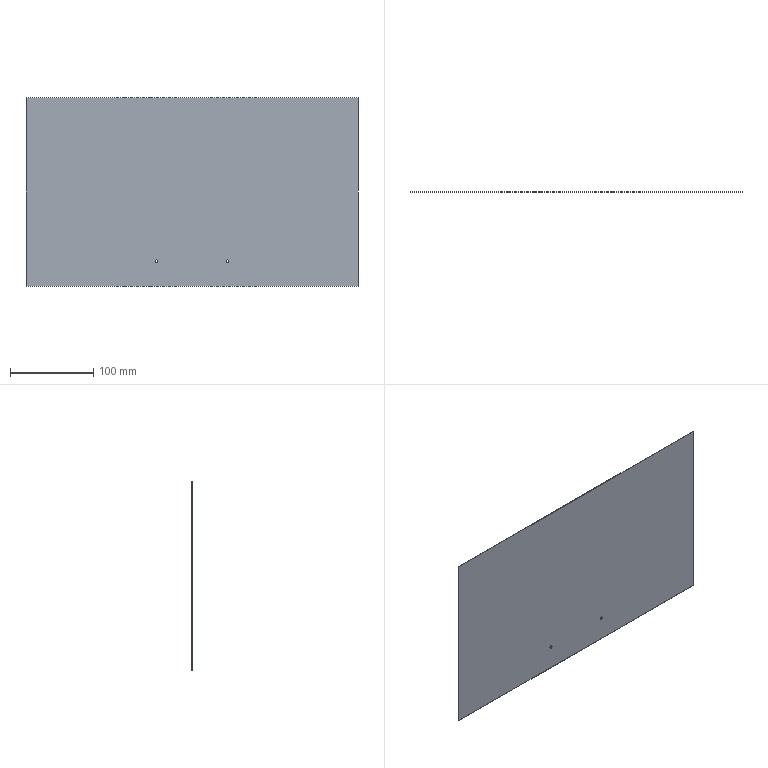Part | SolidWorks | features 3DProfileFeature 1, FlatPattern 1, HoleWzd 1, SMBaseFlange 1, SheetMetal 1 | 1 solid | 10 faces | box 398 x 0.5 x 226 mm | volume 44966 mm3 | plane 6 | cylinder 4 | commonest cylinder face diameters 3.2 x4
STEP:
#1=CARTESIAN_POINT('',(156.5,0.,-194.4));
#2=VERTEX_POINT('',#1);
#3=CARTESIAN_POINT('',(156.5,0.,-197.6));
#4=VERTEX_POINT('',#3);
#5=CARTESIAN_POINT('',(156.5,0.,-196.));
#6=DIRECTION('',(0.,-1.,0.));
#7=DIRECTION('',(0.,0.,-1.));
#8=AXIS2_PLACEMENT_3D('',#5,#6,#7);
#9=CIRCLE('',#8,1.6);
#10=EDGE_CURVE('',#2,#4,#9,.T.);
#11=ORIENTED_EDGE('',*,*,#10,.T.);
#12=CARTESIAN_POINT('',(156.5,0.5,-197.6));
#13=VERTEX_POINT('',#12);
#14=CARTESIAN_POINT('',(156.5,0.5,-197.6));
#15=DIRECTION('',(0.,1.,0.));
#16=VECTOR('',#15,1000.);
#17=LINE('',#14,#16);
#18=EDGE_CURVE('',#4,#13,#17,.T.);
#19=ORIENTED_EDGE('',*,*,#18,.T.);
#20=CARTESIAN_POINT('',(156.5,0.5,-194.4));
#21=VERTEX_POINT('',#20);
#22=CARTESIAN_POINT('',(156.5,0.5,-196.));
#23=DIRECTION('',(0.,1.,0.));
#24=DIRECTION('',(0.,0.,1.));
#25=AXIS2_PLACEMENT_3D('',#22,#23,#24);
#26=CIRCLE('',#25,1.6);
#27=EDGE_CURVE('',#13,#21,#26,.T.);
#28=ORIENTED_EDGE('',*,*,#27,.T.);
#29=CARTESIAN_POINT('',(156.5,0.5,-194.4));
#30=DIRECTION('',(0.,1.,0.));
#31=VECTOR('',#30,1000.);
#32=LINE('',#29,#31);
#33=EDGE_CURVE('',#2,#21,#32,.T.);
#34=ORIENTED_EDGE('',*,*,#33,.F.);
#35=EDGE_LOOP('',(#11,#19,#28,#34));
#36=FACE_OUTER_BOUND('',#35,.T.);
#37=CARTESIAN_POINT('',(156.5,0.5,-196.));
#38=DIRECTION('',(0.,1.,0.));
#39=DIRECTION('',(0.,0.,1.));
#40=AXIS2_PLACEMENT_3D('',#37,#38,#39);
#41=CYLINDRICAL_SURFACE('',#40,1.6);
#42=ADVANCED_FACE('',(#36),#41,.F.);
#43=CARTESIAN_POINT('',(241.5,0.,-194.4));
#44=VERTEX_POINT('',#43);
#45=CARTESIAN_POINT('',(241.5,0.,-197.6));
#46=VERTEX_POINT('',#45);
#47=CARTESIAN_POINT('',(241.5,0.,-196.));
#48=DIRECTION('',(0.,-1.,0.));
#49=DIRECTION('',(0.,0.,-1.));
#50=AXIS2_PLACEMENT_3D('',#47,#48,#49);
#51=CIRCLE('',#50,1.6);
#52=EDGE_CURVE('',#44,#46,#51,.T.);
#53=ORIENTED_EDGE('',*,*,#52,.T.);
#54=CARTESIAN_POINT('',(241.5,0.5,-197.6));
#55=VERTEX_POINT('',#54);
#56=CARTESIAN_POINT('',(241.5,0.5,-197.6));
#57=DIRECTION('',(0.,1.,0.));
#58=VECTOR('',#57,1000.);
#59=LINE('',#56,#58);
#60=EDGE_CURVE('',#46,#55,#59,.T.);
#61=ORIENTED_EDGE('',*,*,#60,.T.);
#62=CARTESIAN_POINT('',(241.5,0.5,-194.4));
#63=VERTEX_POINT('',#62);
#64=CARTESIAN_POINT('',(241.5,0.5,-196.));
#65=DIRECTION('',(0.,1.,0.));
#66=DIRECTION('',(0.,0.,1.));
#67=AXIS2_PLACEMENT_3D('',#64,#65,#66);
#68=CIRCLE('',#67,1.6);
#69=EDGE_CURVE('',#55,#63,#68,.T.);
#70=ORIENTED_EDGE('',*,*,#69,.T.);
#71=CARTESIAN_POINT('',(241.5,0.5,-194.4));
#72=DIRECTION('',(0.,1.,0.));
#73=VECTOR('',#72,1000.);
#74=LINE('',#71,#73);
#75=EDGE_CURVE('',#44,#63,#74,.T.);
#76=ORIENTED_EDGE('',*,*,#75,.F.);
#77=EDGE_LOOP('',(#53,#61,#70,#76));
#78=FACE_OUTER_BOUND('',#77,.T.);
#79=CARTESIAN_POINT('',(241.5,0.5,-196.));
#80=DIRECTION('',(0.,1.,0.));
#81=DIRECTION('',(0.,0.,1.));
#82=AXIS2_PLACEMENT_3D('',#79,#80,#81);
#83=CYLINDRICAL_SURFACE('',#82,1.6);
#84=ADVANCED_FACE('',(#78),#83,.F.);
#85=CARTESIAN_POINT('',(0.,0.,-226.));
#86=VERTEX_POINT('',#85);
#87=CARTESIAN_POINT('',(0.,0.,0.));
#88=VERTEX_POINT('',#87);
#89=CARTESIAN_POINT('',(0.,0.,0.));
#90=DIRECTION('',(0.,0.,1.));
#91=VECTOR('',#90,1000.);
#92=LINE('',#89,#91);
#93=EDGE_CURVE('',#86,#88,#92,.T.);
#94=ORIENTED_EDGE('',*,*,#93,.T.);
#95=CARTESIAN_POINT('',(0.,0.5,0.));
#96=VERTEX_POINT('',#95);
#97=CARTESIAN_POINT('',(0.,0.5,0.));
#98=DIRECTION('',(0.,-1.,0.));
#99=VECTOR('',#98,1000.);
#100=LINE('',#97,#99);
#101=EDGE_CURVE('',#96,#88,#100,.T.);
#102=ORIENTED_EDGE('',*,*,#101,.F.);
#103=CARTESIAN_POINT('',(0.,0.5,-226.));
#104=VERTEX_POINT('',#103);
#105=CARTESIAN_POINT('',(0.,0.5,0.));
#106=DIRECTION('',(0.,0.,1.));
#107=VECTOR('',#106,1000.);
#108=LINE('',#105,#107);
#109=EDGE_CURVE('',#104,#96,#108,.T.);
#110=ORIENTED_EDGE('',*,*,#109,.F.);
#111=CARTESIAN_POINT('',(0.,0.5,-226.));
#112=DIRECTION('',(0.,-1.,0.));
#113=VECTOR('',#112,1000.);
#114=LINE('',#111,#113);
#115=EDGE_CURVE('',#104,#86,#114,.T.);
#116=ORIENTED_EDGE('',*,*,#115,.T.);
#117=EDGE_LOOP('',(#94,#102,#110,#116));
#118=FACE_OUTER_BOUND('',#117,.T.);
#119=CARTESIAN_POINT('',(0.,0.5,0.));
#120=DIRECTION('',(1.,0.,0.));
#121=DIRECTION('',(0.,0.,-1.));
#122=AXIS2_PLACEMENT_3D('',#119,#120,#121);
#123=PLANE('',#122);
#124=ADVANCED_FACE('',(#118),#123,.F.);
#125=CARTESIAN_POINT('',(398.,0.,0.));
#126=VERTEX_POINT('',#125);
#127=CARTESIAN_POINT('',(0.,0.,0.));
#128=DIRECTION('',(1.,0.,0.));
#129=VECTOR('',#128,1000.);
#130=LINE('',#127,#129);
#131=EDGE_CURVE('',#88,#126,#130,.T.);
#132=ORIENTED_EDGE('',*,*,#131,.T.);
#133=CARTESIAN_POINT('',(398.,0.5,0.));
#134=VERTEX_POINT('',#133);
#135=CARTESIAN_POINT('',(398.,0.5,0.));
#136=DIRECTION('',(0.,-1.,0.));
#137=VECTOR('',#136,1000.);
#138=LINE('',#135,#137);
#139=EDGE_CURVE('',#134,#126,#138,.T.);
#140=ORIENTED_EDGE('',*,*,#139,.F.);
#141=CARTESIAN_POINT('',(0.,0.5,0.));
#142=DIRECTION('',(1.,0.,0.));
#143=VECTOR('',#142,1000.);
#144=LINE('',#141,#143);
#145=EDGE_CURVE('',#96,#134,#144,.T.);
#146=ORIENTED_EDGE('',*,*,#145,.F.);
#147=ORIENTED_EDGE('',*,*,#101,.T.);
#148=EDGE_LOOP('',(#132,#140,#146,#147));
#149=FACE_OUTER_BOUND('',#148,.T.);
#150=CARTESIAN_POINT('',(0.,0.5,0.));
#151=DIRECTION('',(0.,0.,-1.));
#152=DIRECTION('',(-1.,0.,0.));
#153=AXIS2_PLACEMENT_3D('',#150,#151,#152);
#154=PLANE('',#153);
#155=ADVANCED_FACE('',(#149),#154,.F.);
#156=CARTESIAN_POINT('',(398.,0.,-226.));
#157=VERTEX_POINT('',#156);
#158=CARTESIAN_POINT('',(398.,0.,0.));
#159=DIRECTION('',(0.,0.,-1.));
#160=VECTOR('',#159,1000.);
#161=LINE('',#158,#160);
#162=EDGE_CURVE('',#126,#157,#161,.T.);
#163=ORIENTED_EDGE('',*,*,#162,.T.);
#164=CARTESIAN_POINT('',(398.,0.5,-226.));
#165=VERTEX_POINT('',#164);
#166=CARTESIAN_POINT('',(398.,0.5,-226.));
#167=DIRECTION('',(0.,-1.,0.));
#168=VECTOR('',#167,1000.);
#169=LINE('',#166,#168);
#170=EDGE_CURVE('',#165,#157,#169,.T.);
#171=ORIENTED_EDGE('',*,*,#170,.F.);
#172=CARTESIAN_POINT('',(398.,0.5,0.));
#173=DIRECTION('',(0.,0.,-1.));
#174=VECTOR('',#173,1000.);
#175=LINE('',#172,#174);
#176=EDGE_CURVE('',#134,#165,#175,.T.);
#177=ORIENTED_EDGE('',*,*,#176,.F.);
#178=ORIENTED_EDGE('',*,*,#139,.T.);
#179=EDGE_LOOP('',(#163,#171,#177,#178));
#180=FACE_OUTER_BOUND('',#179,.T.);
#181=CARTESIAN_POINT('',(398.,0.5,0.));
#182=DIRECTION('',(-1.,0.,0.));
#183=DIRECTION('',(0.,0.,1.));
#184=AXIS2_PLACEMENT_3D('',#181,#182,#183);
#185=PLANE('',#184);
#186=ADVANCED_FACE('',(#180),#185,.F.);
#187=CARTESIAN_POINT('',(0.,0.,-226.));
#188=DIRECTION('',(-1.,0.,0.));
#189=VECTOR('',#188,1000.);
#190=LINE('',#187,#189);
#191=EDGE_CURVE('',#157,#86,#190,.T.);
#192=ORIENTED_EDGE('',*,*,#191,.T.);
#193=ORIENTED_EDGE('',*,*,#115,.F.);
#194=CARTESIAN_POINT('',(0.,0.5,-226.));
#195=DIRECTION('',(-1.,0.,0.));
#196=VECTOR('',#195,1000.);
#197=LINE('',#194,#196);
#198=EDGE_CURVE('',#165,#104,#197,.T.);
#199=ORIENTED_EDGE('',*,*,#198,.F.);
#200=ORIENTED_EDGE('',*,*,#170,.T.);
#201=EDGE_LOOP('',(#192,#193,#199,#200));
#202=FACE_OUTER_BOUND('',#201,.T.);
#203=CARTESIAN_POINT('',(0.,0.5,-226.));
#204=DIRECTION('',(0.,0.,1.));
#205=DIRECTION('',(1.,0.,0.));
#206=AXIS2_PLACEMENT_3D('',#203,#204,#205);
#207=PLANE('',#206);
#208=ADVANCED_FACE('',(#202),#207,.F.);
#209=CARTESIAN_POINT('',(156.5,0.5,-196.));
#210=DIRECTION('',(0.,1.,0.));
#211=DIRECTION('',(0.,0.,1.));
#212=AXIS2_PLACEMENT_3D('',#209,#210,#211);
#213=CIRCLE('',#212,1.6);
#214=EDGE_CURVE('',#21,#13,#213,.T.);
#215=ORIENTED_EDGE('',*,*,#214,.F.);
#216=ORIENTED_EDGE('',*,*,#27,.F.);
#217=EDGE_LOOP('',(#215,#216));
#218=FACE_BOUND('',#217,.T.);
#219=CARTESIAN_POINT('',(241.5,0.5,-196.));
#220=DIRECTION('',(0.,1.,0.));
#221=DIRECTION('',(0.,0.,1.));
#222=AXIS2_PLACEMENT_3D('',#219,#220,#221);
#223=CIRCLE('',#222,1.6);
#224=EDGE_CURVE('',#63,#55,#223,.T.);
#225=ORIENTED_EDGE('',*,*,#224,.F.);
#226=ORIENTED_EDGE('',*,*,#69,.F.);
#227=EDGE_LOOP('',(#225,#226));
#228=FACE_BOUND('',#227,.T.);
#229=ORIENTED_EDGE('',*,*,#109,.T.);
#230=ORIENTED_EDGE('',*,*,#145,.T.);
#231=ORIENTED_EDGE('',*,*,#176,.T.);
#232=ORIENTED_EDGE('',*,*,#198,.T.);
#233=EDGE_LOOP('',(#229,#230,#231,#232));
#234=FACE_OUTER_BOUND('',#233,.T.);
#235=CARTESIAN_POINT('',(0.,0.5,-226.));
#236=DIRECTION('',(0.,-1.,0.));
#237=DIRECTION('',(0.,0.,-1.));
#238=AXIS2_PLACEMENT_3D('',#235,#236,#237);
#239=PLANE('',#238);
#240=ADVANCED_FACE('',(#218,#228,#234),#239,.F.);
#241=ORIENTED_EDGE('',*,*,#10,.F.);
#242=CARTESIAN_POINT('',(156.5,0.,-196.));
#243=DIRECTION('',(0.,-1.,0.));
#244=DIRECTION('',(0.,0.,-1.));
#245=AXIS2_PLACEMENT_3D('',#242,#243,#244);
#246=CIRCLE('',#245,1.6);
#247=EDGE_CURVE('',#4,#2,#246,.T.);
#248=ORIENTED_EDGE('',*,*,#247,.F.);
#249=EDGE_LOOP('',(#241,#248));
#250=FACE_BOUND('',#249,.T.);
#251=ORIENTED_EDGE('',*,*,#52,.F.);
#252=CARTESIAN_POINT('',(241.5,0.,-196.));
#253=DIRECTION('',(0.,-1.,0.));
#254=DIRECTION('',(0.,0.,-1.));
#255=AXIS2_PLACEMENT_3D('',#252,#253,#254);
#256=CIRCLE('',#255,1.6);
#257=EDGE_CURVE('',#46,#44,#256,.T.);
#258=ORIENTED_EDGE('',*,*,#257,.F.);
#259=EDGE_LOOP('',(#251,#258));
#260=FACE_BOUND('',#259,.T.);
#261=ORIENTED_EDGE('',*,*,#93,.F.);
#262=ORIENTED_EDGE('',*,*,#191,.F.);
#263=ORIENTED_EDGE('',*,*,#162,.F.);
#264=ORIENTED_EDGE('',*,*,#131,.F.);
#265=EDGE_LOOP('',(#261,#262,#263,#264));
#266=FACE_OUTER_BOUND('',#265,.T.);
#267=CARTESIAN_POINT('',(0.,0.,-226.));
#268=DIRECTION('',(0.,-1.,0.));
#269=DIRECTION('',(0.,0.,-1.));
#270=AXIS2_PLACEMENT_3D('',#267,#268,#269);
#271=PLANE('',#270);
#272=ADVANCED_FACE('',(#250,#260,#266),#271,.T.);
#273=ORIENTED_EDGE('',*,*,#60,.F.);
#274=ORIENTED_EDGE('',*,*,#257,.T.);
#275=ORIENTED_EDGE('',*,*,#75,.T.);
#276=ORIENTED_EDGE('',*,*,#224,.T.);
#277=EDGE_LOOP('',(#273,#274,#275,#276));
#278=FACE_OUTER_BOUND('',#277,.T.);
#279=CARTESIAN_POINT('',(241.5,0.5,-196.));
#280=DIRECTION('',(0.,1.,0.));
#281=DIRECTION('',(0.,0.,1.));
#282=AXIS2_PLACEMENT_3D('',#279,#280,#281);
#283=CYLINDRICAL_SURFACE('',#282,1.6);
#284=ADVANCED_FACE('',(#278),#283,.F.);
#285=ORIENTED_EDGE('',*,*,#18,.F.);
#286=ORIENTED_EDGE('',*,*,#247,.T.);
#287=ORIENTED_EDGE('',*,*,#33,.T.);
#288=ORIENTED_EDGE('',*,*,#214,.T.);
#289=EDGE_LOOP('',(#285,#286,#287,#288));
#290=FACE_OUTER_BOUND('',#289,.T.);
#291=CARTESIAN_POINT('',(156.5,0.5,-196.));
#292=DIRECTION('',(0.,1.,0.));
#293=DIRECTION('',(0.,0.,1.));
#294=AXIS2_PLACEMENT_3D('',#291,#292,#293);
#295=CYLINDRICAL_SURFACE('',#294,1.6);
#296=ADVANCED_FACE('',(#290),#295,.F.);
#297=CLOSED_SHELL('',(#42,#84,#124,#155,#186,#208,#240,#272,#284,#296));
#298=MANIFOLD_SOLID_BREP('',#297);
#299=CARTESIAN_POINT('',(0.,0.,0.));
#300=DIRECTION('',(0.,0.,1.));
#301=DIRECTION('',(1.,0.,0.));
#302=AXIS2_PLACEMENT_3D('',#299,#300,#301);
#303=(LENGTH_UNIT()NAMED_UNIT(*)SI_UNIT(.MILLI.,.METRE.));
#304=UNCERTAINTY_MEASURE_WITH_UNIT(LENGTH_MEASURE(0.00001),#303,'','');
#305=(NAMED_UNIT(*)PLANE_ANGLE_UNIT()SI_UNIT($,.RADIAN.));
#306=(NAMED_UNIT(*)SI_UNIT($,.STERADIAN.)SOLID_ANGLE_UNIT());
#307=(GEOMETRIC_REPRESENTATION_CONTEXT(3)GLOBAL_UNCERTAINTY_ASSIGNED_CONTEXT((#304))GLOBAL_UNIT_ASSIGNED_CONTEXT((#303,#305,#306))REPRESENTATION_CONTEXT('',''));
#308=ADVANCED_BREP_SHAPE_REPRESENTATION('',(#298,#302),#307);